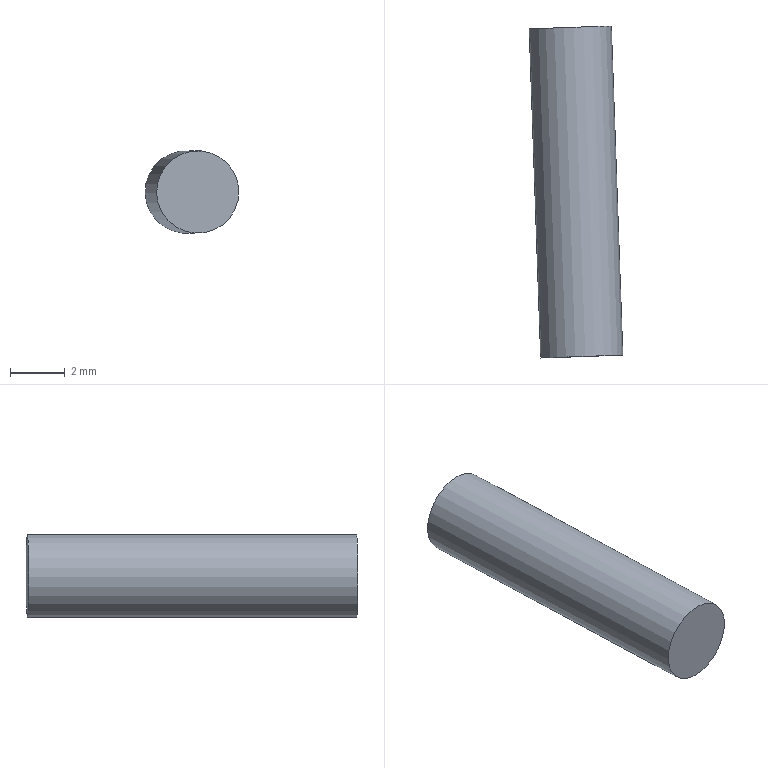Part | NX | features solid 2 | 1 solid | 3 faces | box 3.417 x 12.097 x 3 mm | volume 84.823 mm3 | plane 2 | cylinder 1 | commonest cylinder face diameters 3 x1
STEP:
#1=CARTESIAN_POINT('',(2368.896,-802.015,828.769));
#2=VERTEX_POINT('',#1);
#3=CARTESIAN_POINT('',(2367.398,-802.068,828.716));
#4=DIRECTION('',(-0.0349,0.9994,0.));
#5=DIRECTION('',(0.9988,0.03487,0.0349));
#6=AXIS2_PLACEMENT_3D('',#3,#4,#5);
#7=CIRCLE('',#6,1.5);
#8=EDGE_CURVE('',#2,#2,#7,.T.);
#9=ORIENTED_EDGE('',*,*,#8,.T.);
#10=EDGE_LOOP('',(#9));
#11=FACE_BOUND('',#10,.T.);
#12=CARTESIAN_POINT('',(2367.398,-802.068,828.716));
#13=DIRECTION('',(-0.0349,0.9994,0.));
#14=DIRECTION('',(0.9994,0.0349,0.));
#15=AXIS2_PLACEMENT_3D('',#12,#13,#14);
#16=PLANE('',#15);
#17=ADVANCED_FACE('',(#11),#16,.T.);
#18=CARTESIAN_POINT('',(2369.315,-814.008,828.769));
#19=VERTEX_POINT('',#18);
#20=CARTESIAN_POINT('',(2367.817,-814.06,828.716));
#21=DIRECTION('',(0.0349,-0.9994,0.));
#22=DIRECTION('',(0.9988,0.03487,0.0349));
#23=AXIS2_PLACEMENT_3D('',#20,#21,#22);
#24=CIRCLE('',#23,1.5);
#25=EDGE_CURVE('',#19,#19,#24,.T.);
#26=ORIENTED_EDGE('',*,*,#25,.T.);
#27=EDGE_LOOP('',(#26));
#28=FACE_BOUND('',#27,.T.);
#29=CARTESIAN_POINT('',(2367.817,-814.06,828.716));
#30=DIRECTION('',(0.0349,-0.9994,0.));
#31=DIRECTION('',(-0.9994,-0.0349,0.));
#32=AXIS2_PLACEMENT_3D('',#29,#30,#31);
#33=PLANE('',#32);
#34=ADVANCED_FACE('',(#28),#33,.T.);
#35=ORIENTED_EDGE('',*,*,#8,.F.);
#36=EDGE_LOOP('',(#35));
#37=FACE_BOUND('',#36,.T.);
#38=ORIENTED_EDGE('',*,*,#25,.F.);
#39=EDGE_LOOP('',(#38));
#40=FACE_BOUND('',#39,.T.);
#41=CARTESIAN_POINT('',(2367.817,-814.06,828.716));
#42=DIRECTION('',(-0.0349,0.9994,0.));
#43=DIRECTION('',(0.9988,0.03487,0.0349));
#44=AXIS2_PLACEMENT_3D('',#41,#42,#43);
#45=CYLINDRICAL_SURFACE('',#44,1.5);
#46=ADVANCED_FACE('',(#37,#40),#45,.T.);
#47=CLOSED_SHELL('',(#17,#34,#46));
#48=MANIFOLD_SOLID_BREP('',#47);
#49=(LENGTH_UNIT()NAMED_UNIT(*)SI_UNIT(.MILLI.,.METRE.));
#50=UNCERTAINTY_MEASURE_WITH_UNIT(LENGTH_MEASURE(0.00001),#49,'','');
#51=(NAMED_UNIT(*)PLANE_ANGLE_UNIT()SI_UNIT($,.RADIAN.));
#52=(NAMED_UNIT(*)SI_UNIT($,.STERADIAN.)SOLID_ANGLE_UNIT());
#53=(GEOMETRIC_REPRESENTATION_CONTEXT(3)GLOBAL_UNCERTAINTY_ASSIGNED_CONTEXT((#50))GLOBAL_UNIT_ASSIGNED_CONTEXT((#49,#51,#52))REPRESENTATION_CONTEXT('',''));
#54=ADVANCED_BREP_SHAPE_REPRESENTATION('',(#48),#53);